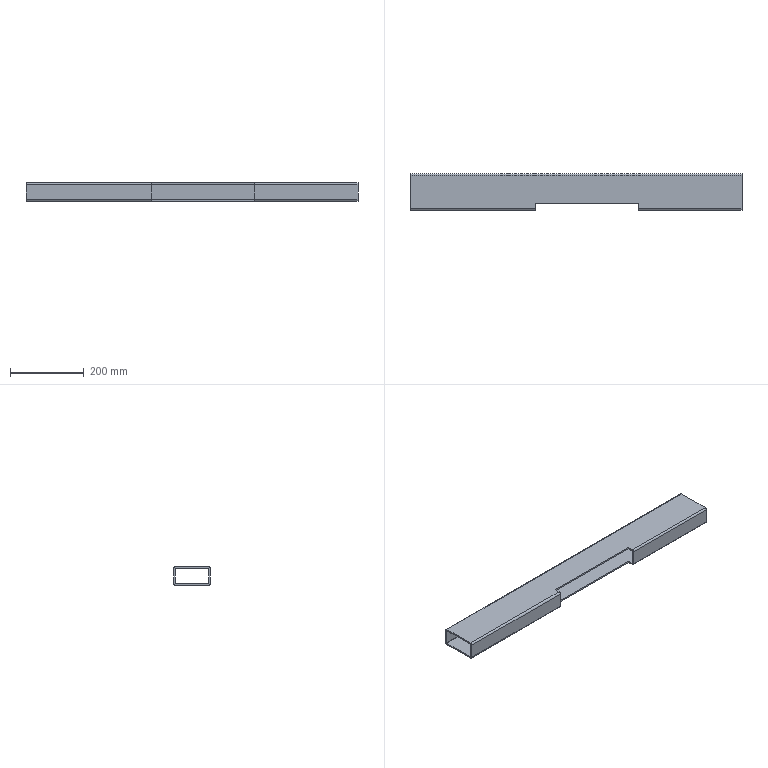Part | SolidWorks | features BaseBody 1 | 1 solid | 28 faces | box 900 x 100 x 50 mm | volume 914903 mm3 | plane 16 | cylinder 12 | commonest cylinder face diameters 2 x6 10 x6
STEP:
#1=CARTESIAN_POINT('',(-110.,-50.,20.));
#2=VERTEX_POINT('',#1);
#3=CARTESIAN_POINT('',(-450.,-50.,20.));
#4=VERTEX_POINT('',#3);
#5=CARTESIAN_POINT('',(450.,-50.,20.));
#6=DIRECTION('',(-1.,0.,0.));
#7=VECTOR('',#6,1000.);
#8=LINE('',#5,#7);
#9=EDGE_CURVE('',#2,#4,#8,.T.);
#10=ORIENTED_EDGE('',*,*,#9,.F.);
#11=CARTESIAN_POINT('',(-110.,-45.,25.));
#12=VERTEX_POINT('',#11);
#13=CARTESIAN_POINT('',(-110.,-45.,20.));
#14=DIRECTION('',(-1.,0.,0.));
#15=DIRECTION('',(0.,-1.,0.));
#16=AXIS2_PLACEMENT_3D('',#13,#14,#15);
#17=CIRCLE('',#16,5.);
#18=EDGE_CURVE('',#2,#12,#17,.T.);
#19=ORIENTED_EDGE('',*,*,#18,.T.);
#20=CARTESIAN_POINT('',(-450.,-45.,25.));
#21=VERTEX_POINT('',#20);
#22=CARTESIAN_POINT('',(450.,-45.,25.));
#23=DIRECTION('',(-1.,0.,0.));
#24=VECTOR('',#23,1000.);
#25=LINE('',#22,#24);
#26=EDGE_CURVE('',#12,#21,#25,.T.);
#27=ORIENTED_EDGE('',*,*,#26,.T.);
#28=CARTESIAN_POINT('',(-450.,-45.,20.));
#29=DIRECTION('',(1.,0.,0.));
#30=DIRECTION('',(0.,0.,-1.));
#31=AXIS2_PLACEMENT_3D('',#28,#29,#30);
#32=CIRCLE('',#31,5.);
#33=EDGE_CURVE('',#21,#4,#32,.T.);
#34=ORIENTED_EDGE('',*,*,#33,.T.);
#35=EDGE_LOOP('',(#10,#19,#27,#34));
#36=FACE_OUTER_BOUND('',#35,.T.);
#37=CARTESIAN_POINT('',(450.,-45.,20.));
#38=DIRECTION('',(-1.,0.,0.));
#39=DIRECTION('',(0.,0.,1.));
#40=AXIS2_PLACEMENT_3D('',#37,#38,#39);
#41=CYLINDRICAL_SURFACE('',#40,5.);
#42=ADVANCED_FACE('',(#36),#41,.T.);
#43=CARTESIAN_POINT('',(-110.,-50.,-20.));
#44=VERTEX_POINT('',#43);
#45=CARTESIAN_POINT('',(-450.,-50.,-20.));
#46=VERTEX_POINT('',#45);
#47=CARTESIAN_POINT('',(450.,-50.,-20.));
#48=DIRECTION('',(-1.,0.,0.));
#49=VECTOR('',#48,1000.);
#50=LINE('',#47,#49);
#51=EDGE_CURVE('',#44,#46,#50,.T.);
#52=ORIENTED_EDGE('',*,*,#51,.F.);
#53=CARTESIAN_POINT('',(-110.,-50.,-25.));
#54=DIRECTION('',(0.,0.,1.));
#55=VECTOR('',#54,1000.);
#56=LINE('',#53,#55);
#57=EDGE_CURVE('',#44,#2,#56,.T.);
#58=ORIENTED_EDGE('',*,*,#57,.T.);
#59=ORIENTED_EDGE('',*,*,#9,.T.);
#60=CARTESIAN_POINT('',(-450.,-50.,20.));
#61=DIRECTION('',(0.,0.,-1.));
#62=VECTOR('',#61,1000.);
#63=LINE('',#60,#62);
#64=EDGE_CURVE('',#4,#46,#63,.T.);
#65=ORIENTED_EDGE('',*,*,#64,.T.);
#66=EDGE_LOOP('',(#52,#58,#59,#65));
#67=FACE_OUTER_BOUND('',#66,.T.);
#68=CARTESIAN_POINT('',(450.,-50.,20.));
#69=DIRECTION('',(0.,1.,0.));
#70=DIRECTION('',(0.,0.,1.));
#71=AXIS2_PLACEMENT_3D('',#68,#69,#70);
#72=PLANE('',#71);
#73=ADVANCED_FACE('',(#67),#72,.F.);
#74=CARTESIAN_POINT('',(-110.,-45.,-25.));
#75=VERTEX_POINT('',#74);
#76=CARTESIAN_POINT('',(-450.,-45.,-25.));
#77=VERTEX_POINT('',#76);
#78=CARTESIAN_POINT('',(450.,-45.,-25.));
#79=DIRECTION('',(-1.,0.,0.));
#80=VECTOR('',#79,1000.);
#81=LINE('',#78,#80);
#82=EDGE_CURVE('',#75,#77,#81,.T.);
#83=ORIENTED_EDGE('',*,*,#82,.F.);
#84=CARTESIAN_POINT('',(-110.,-45.,-20.));
#85=DIRECTION('',(-1.,0.,0.));
#86=DIRECTION('',(0.,-1.,0.));
#87=AXIS2_PLACEMENT_3D('',#84,#85,#86);
#88=CIRCLE('',#87,5.);
#89=EDGE_CURVE('',#75,#44,#88,.T.);
#90=ORIENTED_EDGE('',*,*,#89,.T.);
#91=ORIENTED_EDGE('',*,*,#51,.T.);
#92=CARTESIAN_POINT('',(-450.,-45.,-20.));
#93=DIRECTION('',(1.,0.,0.));
#94=DIRECTION('',(0.,0.,-1.));
#95=AXIS2_PLACEMENT_3D('',#92,#93,#94);
#96=CIRCLE('',#95,5.);
#97=EDGE_CURVE('',#46,#77,#96,.T.);
#98=ORIENTED_EDGE('',*,*,#97,.T.);
#99=EDGE_LOOP('',(#83,#90,#91,#98));
#100=FACE_OUTER_BOUND('',#99,.T.);
#101=CARTESIAN_POINT('',(450.,-45.,-20.));
#102=DIRECTION('',(-1.,0.,0.));
#103=DIRECTION('',(0.,0.,1.));
#104=AXIS2_PLACEMENT_3D('',#101,#102,#103);
#105=CYLINDRICAL_SURFACE('',#104,5.);
#106=ADVANCED_FACE('',(#100),#105,.T.);
#107=CARTESIAN_POINT('',(-110.,-45.,-21.));
#108=VERTEX_POINT('',#107);
#109=CARTESIAN_POINT('',(-110.,-46.,-20.));
#110=VERTEX_POINT('',#109);
#111=CARTESIAN_POINT('',(-110.,-45.,-20.));
#112=DIRECTION('',(-1.,0.,0.));
#113=DIRECTION('',(0.,-1.,0.));
#114=AXIS2_PLACEMENT_3D('',#111,#112,#113);
#115=CIRCLE('',#114,1.);
#116=EDGE_CURVE('',#108,#110,#115,.T.);
#117=ORIENTED_EDGE('',*,*,#116,.F.);
#118=CARTESIAN_POINT('',(-450.,-45.,-21.));
#119=VERTEX_POINT('',#118);
#120=CARTESIAN_POINT('',(450.,-45.,-21.));
#121=DIRECTION('',(-1.,0.,0.));
#122=VECTOR('',#121,1000.);
#123=LINE('',#120,#122);
#124=EDGE_CURVE('',#108,#119,#123,.T.);
#125=ORIENTED_EDGE('',*,*,#124,.T.);
#126=CARTESIAN_POINT('',(-450.,-46.,-20.));
#127=VERTEX_POINT('',#126);
#128=CARTESIAN_POINT('',(-450.,-45.,-20.));
#129=DIRECTION('',(1.,0.,0.));
#130=DIRECTION('',(0.,0.,-1.));
#131=AXIS2_PLACEMENT_3D('',#128,#129,#130);
#132=CIRCLE('',#131,1.);
#133=EDGE_CURVE('',#127,#119,#132,.T.);
#134=ORIENTED_EDGE('',*,*,#133,.F.);
#135=CARTESIAN_POINT('',(450.,-46.,-20.));
#136=DIRECTION('',(-1.,0.,0.));
#137=VECTOR('',#136,1000.);
#138=LINE('',#135,#137);
#139=EDGE_CURVE('',#110,#127,#138,.T.);
#140=ORIENTED_EDGE('',*,*,#139,.F.);
#141=EDGE_LOOP('',(#117,#125,#134,#140));
#142=FACE_OUTER_BOUND('',#141,.T.);
#143=CARTESIAN_POINT('',(450.,-45.,-20.));
#144=DIRECTION('',(-1.,0.,0.));
#145=DIRECTION('',(0.,0.,1.));
#146=AXIS2_PLACEMENT_3D('',#143,#144,#145);
#147=CYLINDRICAL_SURFACE('',#146,1.);
#148=ADVANCED_FACE('',(#142),#147,.F.);
#149=CARTESIAN_POINT('',(-110.,-46.,20.));
#150=VERTEX_POINT('',#149);
#151=CARTESIAN_POINT('',(-110.,-46.,20.));
#152=DIRECTION('',(0.,0.,1.));
#153=VECTOR('',#152,1000.);
#154=LINE('',#151,#153);
#155=EDGE_CURVE('',#110,#150,#154,.T.);
#156=ORIENTED_EDGE('',*,*,#155,.F.);
#157=ORIENTED_EDGE('',*,*,#139,.T.);
#158=CARTESIAN_POINT('',(-450.,-46.,20.));
#159=VERTEX_POINT('',#158);
#160=CARTESIAN_POINT('',(-450.,-46.,20.));
#161=DIRECTION('',(0.,0.,-1.));
#162=VECTOR('',#161,1000.);
#163=LINE('',#160,#162);
#164=EDGE_CURVE('',#159,#127,#163,.T.);
#165=ORIENTED_EDGE('',*,*,#164,.F.);
#166=CARTESIAN_POINT('',(450.,-46.,20.));
#167=DIRECTION('',(-1.,0.,0.));
#168=VECTOR('',#167,1000.);
#169=LINE('',#166,#168);
#170=EDGE_CURVE('',#150,#159,#169,.T.);
#171=ORIENTED_EDGE('',*,*,#170,.F.);
#172=EDGE_LOOP('',(#156,#157,#165,#171));
#173=FACE_OUTER_BOUND('',#172,.T.);
#174=CARTESIAN_POINT('',(450.,-46.,20.));
#175=DIRECTION('',(0.,1.,0.));
#176=DIRECTION('',(0.,0.,1.));
#177=AXIS2_PLACEMENT_3D('',#174,#175,#176);
#178=PLANE('',#177);
#179=ADVANCED_FACE('',(#173),#178,.T.);
#180=CARTESIAN_POINT('',(-110.,-45.,21.));
#181=VERTEX_POINT('',#180);
#182=CARTESIAN_POINT('',(-110.,-45.,20.));
#183=DIRECTION('',(-1.,0.,0.));
#184=DIRECTION('',(0.,-1.,0.));
#185=AXIS2_PLACEMENT_3D('',#182,#183,#184);
#186=CIRCLE('',#185,1.);
#187=EDGE_CURVE('',#150,#181,#186,.T.);
#188=ORIENTED_EDGE('',*,*,#187,.F.);
#189=ORIENTED_EDGE('',*,*,#170,.T.);
#190=CARTESIAN_POINT('',(-450.,-45.,21.));
#191=VERTEX_POINT('',#190);
#192=CARTESIAN_POINT('',(-450.,-45.,20.));
#193=DIRECTION('',(1.,0.,0.));
#194=DIRECTION('',(0.,0.,-1.));
#195=AXIS2_PLACEMENT_3D('',#192,#193,#194);
#196=CIRCLE('',#195,1.);
#197=EDGE_CURVE('',#191,#159,#196,.T.);
#198=ORIENTED_EDGE('',*,*,#197,.F.);
#199=CARTESIAN_POINT('',(450.,-45.,21.));
#200=DIRECTION('',(-1.,0.,0.));
#201=VECTOR('',#200,1000.);
#202=LINE('',#199,#201);
#203=EDGE_CURVE('',#181,#191,#202,.T.);
#204=ORIENTED_EDGE('',*,*,#203,.F.);
#205=EDGE_LOOP('',(#188,#189,#198,#204));
#206=FACE_OUTER_BOUND('',#205,.T.);
#207=CARTESIAN_POINT('',(450.,-45.,20.));
#208=DIRECTION('',(-1.,0.,0.));
#209=DIRECTION('',(0.,0.,1.));
#210=AXIS2_PLACEMENT_3D('',#207,#208,#209);
#211=CYLINDRICAL_SURFACE('',#210,1.);
#212=ADVANCED_FACE('',(#206),#211,.F.);
#213=CARTESIAN_POINT('',(-450.,45.,-25.));
#214=VERTEX_POINT('',#213);
#215=CARTESIAN_POINT('',(-450.,50.,-20.));
#216=VERTEX_POINT('',#215);
#217=CARTESIAN_POINT('',(-450.,45.,-20.));
#218=DIRECTION('',(1.,0.,0.));
#219=DIRECTION('',(0.,0.,-1.));
#220=AXIS2_PLACEMENT_3D('',#217,#218,#219);
#221=CIRCLE('',#220,5.);
#222=EDGE_CURVE('',#214,#216,#221,.T.);
#223=ORIENTED_EDGE('',*,*,#222,.T.);
#224=CARTESIAN_POINT('',(450.,50.,-20.));
#225=VERTEX_POINT('',#224);
#226=CARTESIAN_POINT('',(450.,50.,-20.));
#227=DIRECTION('',(-1.,0.,0.));
#228=VECTOR('',#227,1000.);
#229=LINE('',#226,#228);
#230=EDGE_CURVE('',#225,#216,#229,.T.);
#231=ORIENTED_EDGE('',*,*,#230,.F.);
#232=CARTESIAN_POINT('',(450.,45.,-25.));
#233=VERTEX_POINT('',#232);
#234=CARTESIAN_POINT('',(450.,45.,-20.));
#235=DIRECTION('',(1.,0.,0.));
#236=DIRECTION('',(0.,0.,-1.));
#237=AXIS2_PLACEMENT_3D('',#234,#235,#236);
#238=CIRCLE('',#237,5.);
#239=EDGE_CURVE('',#233,#225,#238,.T.);
#240=ORIENTED_EDGE('',*,*,#239,.F.);
#241=CARTESIAN_POINT('',(450.,45.,-25.));
#242=DIRECTION('',(-1.,0.,0.));
#243=VECTOR('',#242,1000.);
#244=LINE('',#241,#243);
#245=EDGE_CURVE('',#233,#214,#244,.T.);
#246=ORIENTED_EDGE('',*,*,#245,.T.);
#247=EDGE_LOOP('',(#223,#231,#240,#246));
#248=FACE_OUTER_BOUND('',#247,.T.);
#249=CARTESIAN_POINT('',(450.,45.,-20.));
#250=DIRECTION('',(-1.,0.,0.));
#251=DIRECTION('',(0.,0.,1.));
#252=AXIS2_PLACEMENT_3D('',#249,#250,#251);
#253=CYLINDRICAL_SURFACE('',#252,5.);
#254=ADVANCED_FACE('',(#248),#253,.T.);
#255=CARTESIAN_POINT('',(-450.,50.,20.));
#256=VERTEX_POINT('',#255);
#257=CARTESIAN_POINT('',(-450.,50.,-20.));
#258=DIRECTION('',(0.,0.,1.));
#259=VECTOR('',#258,1000.);
#260=LINE('',#257,#259);
#261=EDGE_CURVE('',#216,#256,#260,.T.);
#262=ORIENTED_EDGE('',*,*,#261,.T.);
#263=CARTESIAN_POINT('',(450.,50.,20.));
#264=VERTEX_POINT('',#263);
#265=CARTESIAN_POINT('',(450.,50.,20.));
#266=DIRECTION('',(-1.,0.,0.));
#267=VECTOR('',#266,1000.);
#268=LINE('',#265,#267);
#269=EDGE_CURVE('',#264,#256,#268,.T.);
#270=ORIENTED_EDGE('',*,*,#269,.F.);
#271=CARTESIAN_POINT('',(450.,50.,-20.));
#272=DIRECTION('',(0.,0.,1.));
#273=VECTOR('',#272,1000.);
#274=LINE('',#271,#273);
#275=EDGE_CURVE('',#225,#264,#274,.T.);
#276=ORIENTED_EDGE('',*,*,#275,.F.);
#277=ORIENTED_EDGE('',*,*,#230,.T.);
#278=EDGE_LOOP('',(#262,#270,#276,#277));
#279=FACE_OUTER_BOUND('',#278,.T.);
#280=CARTESIAN_POINT('',(450.,50.,-20.));
#281=DIRECTION('',(0.,-1.,0.));
#282=DIRECTION('',(0.,0.,-1.));
#283=AXIS2_PLACEMENT_3D('',#280,#281,#282);
#284=PLANE('',#283);
#285=ADVANCED_FACE('',(#279),#284,.F.);
#286=CARTESIAN_POINT('',(-450.,45.,25.));
#287=VERTEX_POINT('',#286);
#288=CARTESIAN_POINT('',(-450.,45.,20.));
#289=DIRECTION('',(1.,0.,0.));
#290=DIRECTION('',(0.,0.,-1.));
#291=AXIS2_PLACEMENT_3D('',#288,#289,#290);
#292=CIRCLE('',#291,5.);
#293=EDGE_CURVE('',#256,#287,#292,.T.);
#294=ORIENTED_EDGE('',*,*,#293,.T.);
#295=CARTESIAN_POINT('',(450.,45.,25.));
#296=VERTEX_POINT('',#295);
#297=CARTESIAN_POINT('',(450.,45.,25.));
#298=DIRECTION('',(-1.,0.,0.));
#299=VECTOR('',#298,1000.);
#300=LINE('',#297,#299);
#301=EDGE_CURVE('',#296,#287,#300,.T.);
#302=ORIENTED_EDGE('',*,*,#301,.F.);
#303=CARTESIAN_POINT('',(450.,45.,20.));
#304=DIRECTION('',(1.,0.,0.));
#305=DIRECTION('',(0.,0.,-1.));
#306=AXIS2_PLACEMENT_3D('',#303,#304,#305);
#307=CIRCLE('',#306,5.);
#308=EDGE_CURVE('',#264,#296,#307,.T.);
#309=ORIENTED_EDGE('',*,*,#308,.F.);
#310=ORIENTED_EDGE('',*,*,#269,.T.);
#311=EDGE_LOOP('',(#294,#302,#309,#310));
#312=FACE_OUTER_BOUND('',#311,.T.);
#313=CARTESIAN_POINT('',(450.,45.,20.));
#314=DIRECTION('',(-1.,0.,0.));
#315=DIRECTION('',(0.,0.,1.));
#316=AXIS2_PLACEMENT_3D('',#313,#314,#315);
#317=CYLINDRICAL_SURFACE('',#316,5.);
#318=ADVANCED_FACE('',(#312),#317,.T.);
#319=ORIENTED_EDGE('',*,*,#26,.F.);
#320=CARTESIAN_POINT('',(-110.,-30.,25.));
#321=VERTEX_POINT('',#320);
#322=CARTESIAN_POINT('',(-110.,-50.,25.));
#323=DIRECTION('',(0.,-1.,0.));
#324=VECTOR('',#323,1000.);
#325=LINE('',#322,#324);
#326=EDGE_CURVE('',#321,#12,#325,.T.);
#327=ORIENTED_EDGE('',*,*,#326,.F.);
#328=CARTESIAN_POINT('',(170.,-30.,25.));
#329=VERTEX_POINT('',#328);
#330=CARTESIAN_POINT('',(170.,-30.,25.));
#331=DIRECTION('',(-1.,0.,0.));
#332=VECTOR('',#331,1000.);
#333=LINE('',#330,#332);
#334=EDGE_CURVE('',#329,#321,#333,.T.);
#335=ORIENTED_EDGE('',*,*,#334,.F.);
#336=CARTESIAN_POINT('',(170.,-45.,25.));
#337=VERTEX_POINT('',#336);
#338=CARTESIAN_POINT('',(170.,-50.,25.));
#339=DIRECTION('',(0.,1.,0.));
#340=VECTOR('',#339,1000.);
#341=LINE('',#338,#340);
#342=EDGE_CURVE('',#337,#329,#341,.T.);
#343=ORIENTED_EDGE('',*,*,#342,.F.);
#344=CARTESIAN_POINT('',(450.,-45.,25.));
#345=VERTEX_POINT('',#344);
#346=CARTESIAN_POINT('',(450.,-45.,25.));
#347=DIRECTION('',(-1.,0.,0.));
#348=VECTOR('',#347,1000.);
#349=LINE('',#346,#348);
#350=EDGE_CURVE('',#345,#337,#349,.T.);
#351=ORIENTED_EDGE('',*,*,#350,.F.);
#352=CARTESIAN_POINT('',(450.,-45.,25.));
#353=DIRECTION('',(0.,-1.,0.));
#354=VECTOR('',#353,1000.);
#355=LINE('',#352,#354);
#356=EDGE_CURVE('',#296,#345,#355,.T.);
#357=ORIENTED_EDGE('',*,*,#356,.F.);
#358=ORIENTED_EDGE('',*,*,#301,.T.);
#359=CARTESIAN_POINT('',(-450.,-45.,25.));
#360=DIRECTION('',(0.,-1.,0.));
#361=VECTOR('',#360,1000.);
#362=LINE('',#359,#361);
#363=EDGE_CURVE('',#287,#21,#362,.T.);
#364=ORIENTED_EDGE('',*,*,#363,.T.);
#365=EDGE_LOOP('',(#319,#327,#335,#343,#351,#357,#358,#364));
#366=FACE_OUTER_BOUND('',#365,.T.);
#367=CARTESIAN_POINT('',(450.,-45.,25.));
#368=DIRECTION('',(0.,0.,-1.));
#369=DIRECTION('',(0.,1.,0.));
#370=AXIS2_PLACEMENT_3D('',#367,#368,#369);
#371=PLANE('',#370);
#372=ADVANCED_FACE('',(#366),#371,.F.);
#373=ORIENTED_EDGE('',*,*,#350,.T.);
#374=CARTESIAN_POINT('',(170.,-50.,20.));
#375=VERTEX_POINT('',#374);
#376=CARTESIAN_POINT('',(170.,-45.,20.));
#377=DIRECTION('',(1.,0.,0.));
#378=DIRECTION('',(0.,1.,0.));
#379=AXIS2_PLACEMENT_3D('',#376,#377,#378);
#380=CIRCLE('',#379,5.);
#381=EDGE_CURVE('',#337,#375,#380,.T.);
#382=ORIENTED_EDGE('',*,*,#381,.T.);
#383=CARTESIAN_POINT('',(450.,-50.,20.));
#384=VERTEX_POINT('',#383);
#385=CARTESIAN_POINT('',(450.,-50.,20.));
#386=DIRECTION('',(-1.,0.,0.));
#387=VECTOR('',#386,1000.);
#388=LINE('',#385,#387);
#389=EDGE_CURVE('',#384,#375,#388,.T.);
#390=ORIENTED_EDGE('',*,*,#389,.F.);
#391=CARTESIAN_POINT('',(450.,-45.,20.));
#392=DIRECTION('',(1.,0.,0.));
#393=DIRECTION('',(0.,0.,-1.));
#394=AXIS2_PLACEMENT_3D('',#391,#392,#393);
#395=CIRCLE('',#394,5.);
#396=EDGE_CURVE('',#345,#384,#395,.T.);
#397=ORIENTED_EDGE('',*,*,#396,.F.);
#398=EDGE_LOOP('',(#373,#382,#390,#397));
#399=FACE_OUTER_BOUND('',#398,.T.);
#400=CARTESIAN_POINT('',(450.,-45.,20.));
#401=DIRECTION('',(-1.,0.,0.));
#402=DIRECTION('',(0.,0.,1.));
#403=AXIS2_PLACEMENT_3D('',#400,#401,#402);
#404=CYLINDRICAL_SURFACE('',#403,5.);
#405=ADVANCED_FACE('',(#399),#404,.T.);
#406=ORIENTED_EDGE('',*,*,#389,.T.);
#407=CARTESIAN_POINT('',(170.,-50.,-20.));
#408=VERTEX_POINT('',#407);
#409=CARTESIAN_POINT('',(170.,-50.,-25.));
#410=DIRECTION('',(0.,0.,1.));
#411=VECTOR('',#410,1000.);
#412=LINE('',#409,#411);
#413=EDGE_CURVE('',#408,#375,#412,.T.);
#414=ORIENTED_EDGE('',*,*,#413,.F.);
#415=CARTESIAN_POINT('',(450.,-50.,-20.));
#416=VERTEX_POINT('',#415);
#417=CARTESIAN_POINT('',(450.,-50.,-20.));
#418=DIRECTION('',(-1.,0.,0.));
#419=VECTOR('',#418,1000.);
#420=LINE('',#417,#419);
#421=EDGE_CURVE('',#416,#408,#420,.T.);
#422=ORIENTED_EDGE('',*,*,#421,.F.);
#423=CARTESIAN_POINT('',(450.,-50.,20.));
#424=DIRECTION('',(0.,0.,-1.));
#425=VECTOR('',#424,1000.);
#426=LINE('',#423,#425);
#427=EDGE_CURVE('',#384,#416,#426,.T.);
#428=ORIENTED_EDGE('',*,*,#427,.F.);
#429=EDGE_LOOP('',(#406,#414,#422,#428));
#430=FACE_OUTER_BOUND('',#429,.T.);
#431=CARTESIAN_POINT('',(450.,-50.,20.));
#432=DIRECTION('',(0.,1.,0.));
#433=DIRECTION('',(0.,0.,1.));
#434=AXIS2_PLACEMENT_3D('',#431,#432,#433);
#435=PLANE('',#434);
#436=ADVANCED_FACE('',(#430),#435,.F.);
#437=ORIENTED_EDGE('',*,*,#421,.T.);
#438=CARTESIAN_POINT('',(170.,-45.,-25.));
#439=VERTEX_POINT('',#438);
#440=CARTESIAN_POINT('',(170.,-45.,-20.));
#441=DIRECTION('',(1.,0.,0.));
#442=DIRECTION('',(0.,1.,0.));
#443=AXIS2_PLACEMENT_3D('',#440,#441,#442);
#444=CIRCLE('',#443,5.);
#445=EDGE_CURVE('',#408,#439,#444,.T.);
#446=ORIENTED_EDGE('',*,*,#445,.T.);
#447=CARTESIAN_POINT('',(450.,-45.,-25.));
#448=VERTEX_POINT('',#447);
#449=CARTESIAN_POINT('',(450.,-45.,-25.));
#450=DIRECTION('',(-1.,0.,0.));
#451=VECTOR('',#450,1000.);
#452=LINE('',#449,#451);
#453=EDGE_CURVE('',#448,#439,#452,.T.);
#454=ORIENTED_EDGE('',*,*,#453,.F.);
#455=CARTESIAN_POINT('',(450.,-45.,-20.));
#456=DIRECTION('',(1.,0.,0.));
#457=DIRECTION('',(0.,0.,-1.));
#458=AXIS2_PLACEMENT_3D('',#455,#456,#457);
#459=CIRCLE('',#458,5.);
#460=EDGE_CURVE('',#416,#448,#459,.T.);
#461=ORIENTED_EDGE('',*,*,#460,.F.);
#462=EDGE_LOOP('',(#437,#446,#454,#461));
#463=FACE_OUTER_BOUND('',#462,.T.);
#464=CARTESIAN_POINT('',(450.,-45.,-20.));
#465=DIRECTION('',(-1.,0.,0.));
#466=DIRECTION('',(0.,0.,1.));
#467=AXIS2_PLACEMENT_3D('',#464,#465,#466);
#468=CYLINDRICAL_SURFACE('',#467,5.);
#469=ADVANCED_FACE('',(#463),#468,.T.);
#470=CARTESIAN_POINT('',(-450.,46.,20.));
#471=VERTEX_POINT('',#470);
#472=CARTESIAN_POINT('',(-450.,45.,21.));
#473=VERTEX_POINT('',#472);
#474=CARTESIAN_POINT('',(-450.,45.,20.));
#475=DIRECTION('',(1.,0.,0.));
#476=DIRECTION('',(0.,0.,-1.));
#477=AXIS2_PLACEMENT_3D('',#474,#475,#476);
#478=CIRCLE('',#477,1.);
#479=EDGE_CURVE('',#471,#473,#478,.T.);
#480=ORIENTED_EDGE('',*,*,#479,.F.);
#481=CARTESIAN_POINT('',(450.,46.,20.));
#482=VERTEX_POINT('',#481);
#483=CARTESIAN_POINT('',(450.,46.,20.));
#484=DIRECTION('',(-1.,0.,0.));
#485=VECTOR('',#484,1000.);
#486=LINE('',#483,#485);
#487=EDGE_CURVE('',#482,#471,#486,.T.);
#488=ORIENTED_EDGE('',*,*,#487,.F.);
#489=CARTESIAN_POINT('',(450.,45.,21.));
#490=VERTEX_POINT('',#489);
#491=CARTESIAN_POINT('',(450.,45.,20.));
#492=DIRECTION('',(1.,0.,0.));
#493=DIRECTION('',(0.,0.,-1.));
#494=AXIS2_PLACEMENT_3D('',#491,#492,#493);
#495=CIRCLE('',#494,1.);
#496=EDGE_CURVE('',#482,#490,#495,.T.);
#497=ORIENTED_EDGE('',*,*,#496,.T.);
#498=CARTESIAN_POINT('',(450.,45.,21.));
#499=DIRECTION('',(-1.,0.,0.));
#500=VECTOR('',#499,1000.);
#501=LINE('',#498,#500);
#502=EDGE_CURVE('',#490,#473,#501,.T.);
#503=ORIENTED_EDGE('',*,*,#502,.T.);
#504=EDGE_LOOP('',(#480,#488,#497,#503));
#505=FACE_OUTER_BOUND('',#504,.T.);
#506=CARTESIAN_POINT('',(450.,45.,20.));
#507=DIRECTION('',(-1.,0.,0.));
#508=DIRECTION('',(0.,0.,1.));
#509=AXIS2_PLACEMENT_3D('',#506,#507,#508);
#510=CYLINDRICAL_SURFACE('',#509,1.);
#511=ADVANCED_FACE('',(#505),#510,.F.);
#512=CARTESIAN_POINT('',(-450.,46.,-20.));
#513=VERTEX_POINT('',#512);
#514=CARTESIAN_POINT('',(-450.,46.,-20.));
#515=DIRECTION('',(0.,0.,1.));
#516=VECTOR('',#515,1000.);
#517=LINE('',#514,#516);
#518=EDGE_CURVE('',#513,#471,#517,.T.);
#519=ORIENTED_EDGE('',*,*,#518,.F.);
#520=CARTESIAN_POINT('',(450.,46.,-20.));
#521=VERTEX_POINT('',#520);
#522=CARTESIAN_POINT('',(450.,46.,-20.));
#523=DIRECTION('',(-1.,0.,0.));
#524=VECTOR('',#523,1000.);
#525=LINE('',#522,#524);
#526=EDGE_CURVE('',#521,#513,#525,.T.);
#527=ORIENTED_EDGE('',*,*,#526,.F.);
#528=CARTESIAN_POINT('',(450.,46.,-20.));
#529=DIRECTION('',(0.,0.,1.));
#530=VECTOR('',#529,1000.);
#531=LINE('',#528,#530);
#532=EDGE_CURVE('',#521,#482,#531,.T.);
#533=ORIENTED_EDGE('',*,*,#532,.T.);
#534=ORIENTED_EDGE('',*,*,#487,.T.);
#535=EDGE_LOOP('',(#519,#527,#533,#534));
#536=FACE_OUTER_BOUND('',#535,.T.);
#537=CARTESIAN_POINT('',(450.,46.,-20.));
#538=DIRECTION('',(0.,-1.,0.));
#539=DIRECTION('',(0.,0.,-1.));
#540=AXIS2_PLACEMENT_3D('',#537,#538,#539);
#541=PLANE('',#540);
#542=ADVANCED_FACE('',(#536),#541,.T.);
#543=CARTESIAN_POINT('',(-450.,45.,-21.));
#544=VERTEX_POINT('',#543);
#545=CARTESIAN_POINT('',(-450.,45.,-20.));
#546=DIRECTION('',(1.,0.,0.));
#547=DIRECTION('',(0.,0.,-1.));
#548=AXIS2_PLACEMENT_3D('',#545,#546,#547);
#549=CIRCLE('',#548,1.);
#550=EDGE_CURVE('',#544,#513,#549,.T.);
#551=ORIENTED_EDGE('',*,*,#550,.F.);
#552=CARTESIAN_POINT('',(450.,45.,-21.));
#553=VERTEX_POINT('',#552);
#554=CARTESIAN_POINT('',(450.,45.,-21.));
#555=DIRECTION('',(-1.,0.,0.));
#556=VECTOR('',#555,1000.);
#557=LINE('',#554,#556);
#558=EDGE_CURVE('',#553,#544,#557,.T.);
#559=ORIENTED_EDGE('',*,*,#558,.F.);
#560=CARTESIAN_POINT('',(450.,45.,-20.));
#561=DIRECTION('',(1.,0.,0.));
#562=DIRECTION('',(0.,0.,-1.));
#563=AXIS2_PLACEMENT_3D('',#560,#561,#562);
#564=CIRCLE('',#563,1.);
#565=EDGE_CURVE('',#553,#521,#564,.T.);
#566=ORIENTED_EDGE('',*,*,#565,.T.);
#567=ORIENTED_EDGE('',*,*,#526,.T.);
#568=EDGE_LOOP('',(#551,#559,#566,#567));
#569=FACE_OUTER_BOUND('',#568,.T.);
#570=CARTESIAN_POINT('',(450.,45.,-20.));
#571=DIRECTION('',(-1.,0.,0.));
#572=DIRECTION('',(0.,0.,1.));
#573=AXIS2_PLACEMENT_3D('',#570,#571,#572);
#574=CYLINDRICAL_SURFACE('',#573,1.);
#575=ADVANCED_FACE('',(#569),#574,.F.);
#576=CARTESIAN_POINT('',(-110.,-30.,-21.));
#577=VERTEX_POINT('',#576);
#578=CARTESIAN_POINT('',(-110.,45.,-21.));
#579=DIRECTION('',(0.,-1.,0.));
#580=VECTOR('',#579,1000.);
#581=LINE('',#578,#580);
#582=EDGE_CURVE('',#577,#108,#581,.T.);
#583=ORIENTED_EDGE('',*,*,#582,.F.);
#584=CARTESIAN_POINT('',(170.,-30.,-21.));
#585=VERTEX_POINT('',#584);
#586=CARTESIAN_POINT('',(450.,-30.,-21.));
#587=DIRECTION('',(-1.,0.,0.));
#588=VECTOR('',#587,1000.);
#589=LINE('',#586,#588);
#590=EDGE_CURVE('',#585,#577,#589,.T.);
#591=ORIENTED_EDGE('',*,*,#590,.F.);
#592=CARTESIAN_POINT('',(170.,-45.,-21.));
#593=VERTEX_POINT('',#592);
#594=CARTESIAN_POINT('',(170.,45.,-21.));
#595=DIRECTION('',(0.,1.,0.));
#596=VECTOR('',#595,1000.);
#597=LINE('',#594,#596);
#598=EDGE_CURVE('',#593,#585,#597,.T.);
#599=ORIENTED_EDGE('',*,*,#598,.F.);
#600=CARTESIAN_POINT('',(450.,-45.,-21.));
#601=VERTEX_POINT('',#600);
#602=CARTESIAN_POINT('',(450.,-45.,-21.));
#603=DIRECTION('',(-1.,0.,0.));
#604=VECTOR('',#603,1000.);
#605=LINE('',#602,#604);
#606=EDGE_CURVE('',#601,#593,#605,.T.);
#607=ORIENTED_EDGE('',*,*,#606,.F.);
#608=CARTESIAN_POINT('',(450.,45.,-21.));
#609=DIRECTION('',(0.,1.,0.));
#610=VECTOR('',#609,1000.);
#611=LINE('',#608,#610);
#612=EDGE_CURVE('',#601,#553,#611,.T.);
#613=ORIENTED_EDGE('',*,*,#612,.T.);
#614=ORIENTED_EDGE('',*,*,#558,.T.);
#615=CARTESIAN_POINT('',(-450.,45.,-21.));
#616=DIRECTION('',(0.,1.,0.));
#617=VECTOR('',#616,1000.);
#618=LINE('',#615,#617);
#619=EDGE_CURVE('',#119,#544,#618,.T.);
#620=ORIENTED_EDGE('',*,*,#619,.F.);
#621=ORIENTED_EDGE('',*,*,#124,.F.);
#622=EDGE_LOOP('',(#583,#591,#599,#607,#613,#614,#620,#621));
#623=FACE_OUTER_BOUND('',#622,.T.);
#624=CARTESIAN_POINT('',(450.,45.,-21.));
#625=DIRECTION('',(0.,0.,1.));
#626=DIRECTION('',(1.,0.,0.));
#627=AXIS2_PLACEMENT_3D('',#624,#625,#626);
#628=PLANE('',#627);
#629=ADVANCED_FACE('',(#623),#628,.T.);
#630=CARTESIAN_POINT('',(170.,-46.,-20.));
#631=VERTEX_POINT('',#630);
#632=CARTESIAN_POINT('',(170.,-45.,-20.));
#633=DIRECTION('',(1.,0.,0.));
#634=DIRECTION('',(0.,1.,0.));
#635=AXIS2_PLACEMENT_3D('',#632,#633,#634);
#636=CIRCLE('',#635,1.);
#637=EDGE_CURVE('',#631,#593,#636,.T.);
#638=ORIENTED_EDGE('',*,*,#637,.F.);
#639=CARTESIAN_POINT('',(450.,-46.,-20.));
#640=VERTEX_POINT('',#639);
#641=CARTESIAN_POINT('',(450.,-46.,-20.));
#642=DIRECTION('',(-1.,0.,0.));
#643=VECTOR('',#642,1000.);
#644=LINE('',#641,#643);
#645=EDGE_CURVE('',#640,#631,#644,.T.);
#646=ORIENTED_EDGE('',*,*,#645,.F.);
#647=CARTESIAN_POINT('',(450.,-45.,-20.));
#648=DIRECTION('',(1.,0.,0.));
#649=DIRECTION('',(0.,0.,-1.));
#650=AXIS2_PLACEMENT_3D('',#647,#648,#649);
#651=CIRCLE('',#650,1.);
#652=EDGE_CURVE('',#640,#601,#651,.T.);
#653=ORIENTED_EDGE('',*,*,#652,.T.);
#654=ORIENTED_EDGE('',*,*,#606,.T.);
#655=EDGE_LOOP('',(#638,#646,#653,#654));
#656=FACE_OUTER_BOUND('',#655,.T.);
#657=CARTESIAN_POINT('',(450.,-45.,-20.));
#658=DIRECTION('',(-1.,0.,0.));
#659=DIRECTION('',(0.,0.,1.));
#660=AXIS2_PLACEMENT_3D('',#657,#658,#659);
#661=CYLINDRICAL_SURFACE('',#660,1.);
#662=ADVANCED_FACE('',(#656),#661,.F.);
#663=CARTESIAN_POINT('',(170.,-46.,20.));
#664=VERTEX_POINT('',#663);
#665=CARTESIAN_POINT('',(170.,-46.,20.));
#666=DIRECTION('',(0.,0.,-1.));
#667=VECTOR('',#666,1000.);
#668=LINE('',#665,#667);
#669=EDGE_CURVE('',#664,#631,#668,.T.);
#670=ORIENTED_EDGE('',*,*,#669,.F.);
#671=CARTESIAN_POINT('',(450.,-46.,20.));
#672=VERTEX_POINT('',#671);
#673=CARTESIAN_POINT('',(450.,-46.,20.));
#674=DIRECTION('',(-1.,0.,0.));
#675=VECTOR('',#674,1000.);
#676=LINE('',#673,#675);
#677=EDGE_CURVE('',#672,#664,#676,.T.);
#678=ORIENTED_EDGE('',*,*,#677,.F.);
#679=CARTESIAN_POINT('',(450.,-46.,20.));
#680=DIRECTION('',(0.,0.,-1.));
#681=VECTOR('',#680,1000.);
#682=LINE('',#679,#681);
#683=EDGE_CURVE('',#672,#640,#682,.T.);
#684=ORIENTED_EDGE('',*,*,#683,.T.);
#685=ORIENTED_EDGE('',*,*,#645,.T.);
#686=EDGE_LOOP('',(#670,#678,#684,#685));
#687=FACE_OUTER_BOUND('',#686,.T.);
#688=CARTESIAN_POINT('',(450.,-46.,20.));
#689=DIRECTION('',(0.,1.,0.));
#690=DIRECTION('',(0.,0.,1.));
#691=AXIS2_PLACEMENT_3D('',#688,#689,#690);
#692=PLANE('',#691);
#693=ADVANCED_FACE('',(#687),#692,.T.);
#694=CARTESIAN_POINT('',(170.,-45.,21.));
#695=VERTEX_POINT('',#694);
#696=CARTESIAN_POINT('',(170.,-45.,20.));
#697=DIRECTION('',(1.,0.,0.));
#698=DIRECTION('',(0.,1.,0.));
#699=AXIS2_PLACEMENT_3D('',#696,#697,#698);
#700=CIRCLE('',#699,1.);
#701=EDGE_CURVE('',#695,#664,#700,.T.);
#702=ORIENTED_EDGE('',*,*,#701,.F.);
#703=CARTESIAN_POINT('',(450.,-45.,21.));
#704=VERTEX_POINT('',#703);
#705=CARTESIAN_POINT('',(450.,-45.,21.));
#706=DIRECTION('',(-1.,0.,0.));
#707=VECTOR('',#706,1000.);
#708=LINE('',#705,#707);
#709=EDGE_CURVE('',#704,#695,#708,.T.);
#710=ORIENTED_EDGE('',*,*,#709,.F.);
#711=CARTESIAN_POINT('',(450.,-45.,20.));
#712=DIRECTION('',(1.,0.,0.));
#713=DIRECTION('',(0.,0.,-1.));
#714=AXIS2_PLACEMENT_3D('',#711,#712,#713);
#715=CIRCLE('',#714,1.);
#716=EDGE_CURVE('',#704,#672,#715,.T.);
#717=ORIENTED_EDGE('',*,*,#716,.T.);
#718=ORIENTED_EDGE('',*,*,#677,.T.);
#719=EDGE_LOOP('',(#702,#710,#717,#718));
#720=FACE_OUTER_BOUND('',#719,.T.);
#721=CARTESIAN_POINT('',(450.,-45.,20.));
#722=DIRECTION('',(-1.,0.,0.));
#723=DIRECTION('',(0.,0.,1.));
#724=AXIS2_PLACEMENT_3D('',#721,#722,#723);
#725=CYLINDRICAL_SURFACE('',#724,1.);
#726=ADVANCED_FACE('',(#720),#725,.F.);
#727=CARTESIAN_POINT('',(-110.,-30.,21.));
#728=VERTEX_POINT('',#727);
#729=CARTESIAN_POINT('',(-110.,-45.,21.));
#730=DIRECTION('',(0.,1.,0.));
#731=VECTOR('',#730,1000.);
#732=LINE('',#729,#731);
#733=EDGE_CURVE('',#181,#728,#732,.T.);
#734=ORIENTED_EDGE('',*,*,#733,.F.);
#735=ORIENTED_EDGE('',*,*,#203,.T.);
#736=CARTESIAN_POINT('',(-450.,-45.,21.));
#737=DIRECTION('',(0.,-1.,0.));
#738=VECTOR('',#737,1000.);
#739=LINE('',#736,#738);
#740=EDGE_CURVE('',#473,#191,#739,.T.);
#741=ORIENTED_EDGE('',*,*,#740,.F.);
#742=ORIENTED_EDGE('',*,*,#502,.F.);
#743=CARTESIAN_POINT('',(450.,-45.,21.));
#744=DIRECTION('',(0.,-1.,0.));
#745=VECTOR('',#744,1000.);
#746=LINE('',#743,#745);
#747=EDGE_CURVE('',#490,#704,#746,.T.);
#748=ORIENTED_EDGE('',*,*,#747,.T.);
#749=ORIENTED_EDGE('',*,*,#709,.T.);
#750=CARTESIAN_POINT('',(170.,-30.,21.));
#751=VERTEX_POINT('',#750);
#752=CARTESIAN_POINT('',(170.,-45.,21.));
#753=DIRECTION('',(0.,-1.,0.));
#754=VECTOR('',#753,1000.);
#755=LINE('',#752,#754);
#756=EDGE_CURVE('',#751,#695,#755,.T.);
#757=ORIENTED_EDGE('',*,*,#756,.F.);
#758=CARTESIAN_POINT('',(450.,-30.,21.));
#759=DIRECTION('',(1.,0.,0.));
#760=VECTOR('',#759,1000.);
#761=LINE('',#758,#760);
#762=EDGE_CURVE('',#728,#751,#761,.T.);
#763=ORIENTED_EDGE('',*,*,#762,.F.);
#764=EDGE_LOOP('',(#734,#735,#741,#742,#748,#749,#757,#763));
#765=FACE_OUTER_BOUND('',#764,.T.);
#766=CARTESIAN_POINT('',(450.,-45.,21.));
#767=DIRECTION('',(0.,0.,-1.));
#768=DIRECTION('',(0.,1.,0.));
#769=AXIS2_PLACEMENT_3D('',#766,#767,#768);
#770=PLANE('',#769);
#771=ADVANCED_FACE('',(#765),#770,.T.);
#772=CARTESIAN_POINT('',(170.,-30.,-25.));
#773=VERTEX_POINT('',#772);
#774=CARTESIAN_POINT('',(-110.,-30.,-25.));
#775=VERTEX_POINT('',#774);
#776=CARTESIAN_POINT('',(170.,-30.,-25.));
#777=DIRECTION('',(-1.,0.,0.));
#778=VECTOR('',#777,1000.);
#779=LINE('',#776,#778);
#780=EDGE_CURVE('',#773,#775,#779,.T.);
#781=ORIENTED_EDGE('',*,*,#780,.T.);
#782=CARTESIAN_POINT('',(-110.,-50.,-25.));
#783=DIRECTION('',(0.,-1.,0.));
#784=VECTOR('',#783,1000.);
#785=LINE('',#782,#784);
#786=EDGE_CURVE('',#775,#75,#785,.T.);
#787=ORIENTED_EDGE('',*,*,#786,.T.);
#788=ORIENTED_EDGE('',*,*,#82,.T.);
#789=CARTESIAN_POINT('',(-450.,45.,-25.));
#790=DIRECTION('',(0.,1.,0.));
#791=VECTOR('',#790,1000.);
#792=LINE('',#789,#791);
#793=EDGE_CURVE('',#77,#214,#792,.T.);
#794=ORIENTED_EDGE('',*,*,#793,.T.);
#795=ORIENTED_EDGE('',*,*,#245,.F.);
#796=CARTESIAN_POINT('',(450.,45.,-25.));
#797=DIRECTION('',(0.,1.,0.));
#798=VECTOR('',#797,1000.);
#799=LINE('',#796,#798);
#800=EDGE_CURVE('',#448,#233,#799,.T.);
#801=ORIENTED_EDGE('',*,*,#800,.F.);
#802=ORIENTED_EDGE('',*,*,#453,.T.);
#803=CARTESIAN_POINT('',(170.,45.,-25.));
#804=DIRECTION('',(0.,1.,0.));
#805=VECTOR('',#804,1000.);
#806=LINE('',#803,#805);
#807=EDGE_CURVE('',#439,#773,#806,.T.);
#808=ORIENTED_EDGE('',*,*,#807,.T.);
#809=EDGE_LOOP('',(#781,#787,#788,#794,#795,#801,#802,#808));
#810=FACE_OUTER_BOUND('',#809,.T.);
#811=CARTESIAN_POINT('',(450.,45.,-25.));
#812=DIRECTION('',(0.,0.,1.));
#813=DIRECTION('',(1.,0.,0.));
#814=AXIS2_PLACEMENT_3D('',#811,#812,#813);
#815=PLANE('',#814);
#816=ADVANCED_FACE('',(#810),#815,.F.);
#817=ORIENTED_EDGE('',*,*,#496,.F.);
#818=ORIENTED_EDGE('',*,*,#532,.F.);
#819=ORIENTED_EDGE('',*,*,#565,.F.);
#820=ORIENTED_EDGE('',*,*,#612,.F.);
#821=ORIENTED_EDGE('',*,*,#652,.F.);
#822=ORIENTED_EDGE('',*,*,#683,.F.);
#823=ORIENTED_EDGE('',*,*,#716,.F.);
#824=ORIENTED_EDGE('',*,*,#747,.F.);
#825=EDGE_LOOP('',(#817,#818,#819,#820,#821,#822,#823,#824));
#826=FACE_BOUND('',#825,.T.);
#827=ORIENTED_EDGE('',*,*,#239,.T.);
#828=ORIENTED_EDGE('',*,*,#275,.T.);
#829=ORIENTED_EDGE('',*,*,#308,.T.);
#830=ORIENTED_EDGE('',*,*,#356,.T.);
#831=ORIENTED_EDGE('',*,*,#396,.T.);
#832=ORIENTED_EDGE('',*,*,#427,.T.);
#833=ORIENTED_EDGE('',*,*,#460,.T.);
#834=ORIENTED_EDGE('',*,*,#800,.T.);
#835=EDGE_LOOP('',(#827,#828,#829,#830,#831,#832,#833,#834));
#836=FACE_OUTER_BOUND('',#835,.T.);
#837=CARTESIAN_POINT('',(450.,45.,-20.));
#838=DIRECTION('',(1.,0.,0.));
#839=DIRECTION('',(0.,0.,-1.));
#840=AXIS2_PLACEMENT_3D('',#837,#838,#839);
#841=PLANE('',#840);
#842=ADVANCED_FACE('',(#826,#836),#841,.T.);
#843=ORIENTED_EDGE('',*,*,#479,.T.);
#844=ORIENTED_EDGE('',*,*,#740,.T.);
#845=ORIENTED_EDGE('',*,*,#197,.T.);
#846=ORIENTED_EDGE('',*,*,#164,.T.);
#847=ORIENTED_EDGE('',*,*,#133,.T.);
#848=ORIENTED_EDGE('',*,*,#619,.T.);
#849=ORIENTED_EDGE('',*,*,#550,.T.);
#850=ORIENTED_EDGE('',*,*,#518,.T.);
#851=EDGE_LOOP('',(#843,#844,#845,#846,#847,#848,#849,#850));
#852=FACE_BOUND('',#851,.T.);
#853=ORIENTED_EDGE('',*,*,#222,.F.);
#854=ORIENTED_EDGE('',*,*,#793,.F.);
#855=ORIENTED_EDGE('',*,*,#97,.F.);
#856=ORIENTED_EDGE('',*,*,#64,.F.);
#857=ORIENTED_EDGE('',*,*,#33,.F.);
#858=ORIENTED_EDGE('',*,*,#363,.F.);
#859=ORIENTED_EDGE('',*,*,#293,.F.);
#860=ORIENTED_EDGE('',*,*,#261,.F.);
#861=EDGE_LOOP('',(#853,#854,#855,#856,#857,#858,#859,#860));
#862=FACE_OUTER_BOUND('',#861,.T.);
#863=CARTESIAN_POINT('',(-450.,45.,-20.));
#864=DIRECTION('',(1.,0.,0.));
#865=DIRECTION('',(0.,0.,-1.));
#866=AXIS2_PLACEMENT_3D('',#863,#864,#865);
#867=PLANE('',#866);
#868=ADVANCED_FACE('',(#852,#862),#867,.F.);
#869=ORIENTED_EDGE('',*,*,#57,.F.);
#870=ORIENTED_EDGE('',*,*,#89,.F.);
#871=ORIENTED_EDGE('',*,*,#786,.F.);
#872=CARTESIAN_POINT('',(-110.,-30.,-25.));
#873=DIRECTION('',(0.,0.,1.));
#874=VECTOR('',#873,1000.);
#875=LINE('',#872,#874);
#876=EDGE_CURVE('',#775,#577,#875,.T.);
#877=ORIENTED_EDGE('',*,*,#876,.T.);
#878=ORIENTED_EDGE('',*,*,#582,.T.);
#879=ORIENTED_EDGE('',*,*,#116,.T.);
#880=ORIENTED_EDGE('',*,*,#155,.T.);
#881=ORIENTED_EDGE('',*,*,#187,.T.);
#882=ORIENTED_EDGE('',*,*,#733,.T.);
#883=CARTESIAN_POINT('',(-110.,-30.,-25.));
#884=DIRECTION('',(0.,0.,1.));
#885=VECTOR('',#884,1000.);
#886=LINE('',#883,#885);
#887=EDGE_CURVE('',#728,#321,#886,.T.);
#888=ORIENTED_EDGE('',*,*,#887,.T.);
#889=ORIENTED_EDGE('',*,*,#326,.T.);
#890=ORIENTED_EDGE('',*,*,#18,.F.);
#891=EDGE_LOOP('',(#869,#870,#871,#877,#878,#879,#880,#881,#882,#888,#889,#890));
#892=FACE_OUTER_BOUND('',#891,.T.);
#893=CARTESIAN_POINT('',(-110.,-50.,-25.));
#894=DIRECTION('',(-1.,0.,0.));
#895=DIRECTION('',(0.,0.,-1.));
#896=AXIS2_PLACEMENT_3D('',#893,#894,#895);
#897=PLANE('',#896);
#898=ADVANCED_FACE('',(#892),#897,.F.);
#899=ORIENTED_EDGE('',*,*,#590,.T.);
#900=ORIENTED_EDGE('',*,*,#876,.F.);
#901=ORIENTED_EDGE('',*,*,#780,.F.);
#902=CARTESIAN_POINT('',(170.,-30.,-25.));
#903=DIRECTION('',(0.,0.,1.));
#904=VECTOR('',#903,1000.);
#905=LINE('',#902,#904);
#906=EDGE_CURVE('',#773,#585,#905,.T.);
#907=ORIENTED_EDGE('',*,*,#906,.T.);
#908=EDGE_LOOP('',(#899,#900,#901,#907));
#909=FACE_OUTER_BOUND('',#908,.T.);
#910=CARTESIAN_POINT('',(170.,-30.,-25.));
#911=DIRECTION('',(0.,1.,0.));
#912=DIRECTION('',(0.,0.,-1.));
#913=AXIS2_PLACEMENT_3D('',#910,#911,#912);
#914=PLANE('',#913);
#915=ADVANCED_FACE('',(#909),#914,.F.);
#916=ORIENTED_EDGE('',*,*,#342,.T.);
#917=CARTESIAN_POINT('',(170.,-30.,-25.));
#918=DIRECTION('',(0.,0.,1.));
#919=VECTOR('',#918,1000.);
#920=LINE('',#917,#919);
#921=EDGE_CURVE('',#751,#329,#920,.T.);
#922=ORIENTED_EDGE('',*,*,#921,.F.);
#923=ORIENTED_EDGE('',*,*,#756,.T.);
#924=ORIENTED_EDGE('',*,*,#701,.T.);
#925=ORIENTED_EDGE('',*,*,#669,.T.);
#926=ORIENTED_EDGE('',*,*,#637,.T.);
#927=ORIENTED_EDGE('',*,*,#598,.T.);
#928=ORIENTED_EDGE('',*,*,#906,.F.);
#929=ORIENTED_EDGE('',*,*,#807,.F.);
#930=ORIENTED_EDGE('',*,*,#445,.F.);
#931=ORIENTED_EDGE('',*,*,#413,.T.);
#932=ORIENTED_EDGE('',*,*,#381,.F.);
#933=EDGE_LOOP('',(#916,#922,#923,#924,#925,#926,#927,#928,#929,#930,#931,#932));
#934=FACE_OUTER_BOUND('',#933,.T.);
#935=CARTESIAN_POINT('',(170.,-50.,-25.));
#936=DIRECTION('',(1.,0.,0.));
#937=DIRECTION('',(0.,0.,1.));
#938=AXIS2_PLACEMENT_3D('',#935,#936,#937);
#939=PLANE('',#938);
#940=ADVANCED_FACE('',(#934),#939,.F.);
#941=ORIENTED_EDGE('',*,*,#762,.T.);
#942=ORIENTED_EDGE('',*,*,#921,.T.);
#943=ORIENTED_EDGE('',*,*,#334,.T.);
#944=ORIENTED_EDGE('',*,*,#887,.F.);
#945=EDGE_LOOP('',(#941,#942,#943,#944));
#946=FACE_OUTER_BOUND('',#945,.T.);
#947=CARTESIAN_POINT('',(170.,-30.,-25.));
#948=DIRECTION('',(0.,1.,0.));
#949=DIRECTION('',(0.,0.,-1.));
#950=AXIS2_PLACEMENT_3D('',#947,#948,#949);
#951=PLANE('',#950);
#952=ADVANCED_FACE('',(#946),#951,.F.);
#953=CLOSED_SHELL('',(#42,#73,#106,#148,#179,#212,#254,#285,#318,#372,#405,#436,#469,#511,#542,#575,#629,#662,#693,#726,#771,#816,#842,#868,#898,#915,#940,#952));
#954=MANIFOLD_SOLID_BREP('',#953);
#955=CARTESIAN_POINT('',(0.,0.,0.));
#956=DIRECTION('',(0.,0.,1.));
#957=DIRECTION('',(1.,0.,0.));
#958=AXIS2_PLACEMENT_3D('',#955,#956,#957);
#959=(LENGTH_UNIT()NAMED_UNIT(*)SI_UNIT(.MILLI.,.METRE.));
#960=UNCERTAINTY_MEASURE_WITH_UNIT(LENGTH_MEASURE(0.00001),#959,'','');
#961=(NAMED_UNIT(*)PLANE_ANGLE_UNIT()SI_UNIT($,.RADIAN.));
#962=(NAMED_UNIT(*)SI_UNIT($,.STERADIAN.)SOLID_ANGLE_UNIT());
#963=(GEOMETRIC_REPRESENTATION_CONTEXT(3)GLOBAL_UNCERTAINTY_ASSIGNED_CONTEXT((#960))GLOBAL_UNIT_ASSIGNED_CONTEXT((#959,#961,#962))REPRESENTATION_CONTEXT('',''));
#964=ADVANCED_BREP_SHAPE_REPRESENTATION('',(#954,#958),#963);